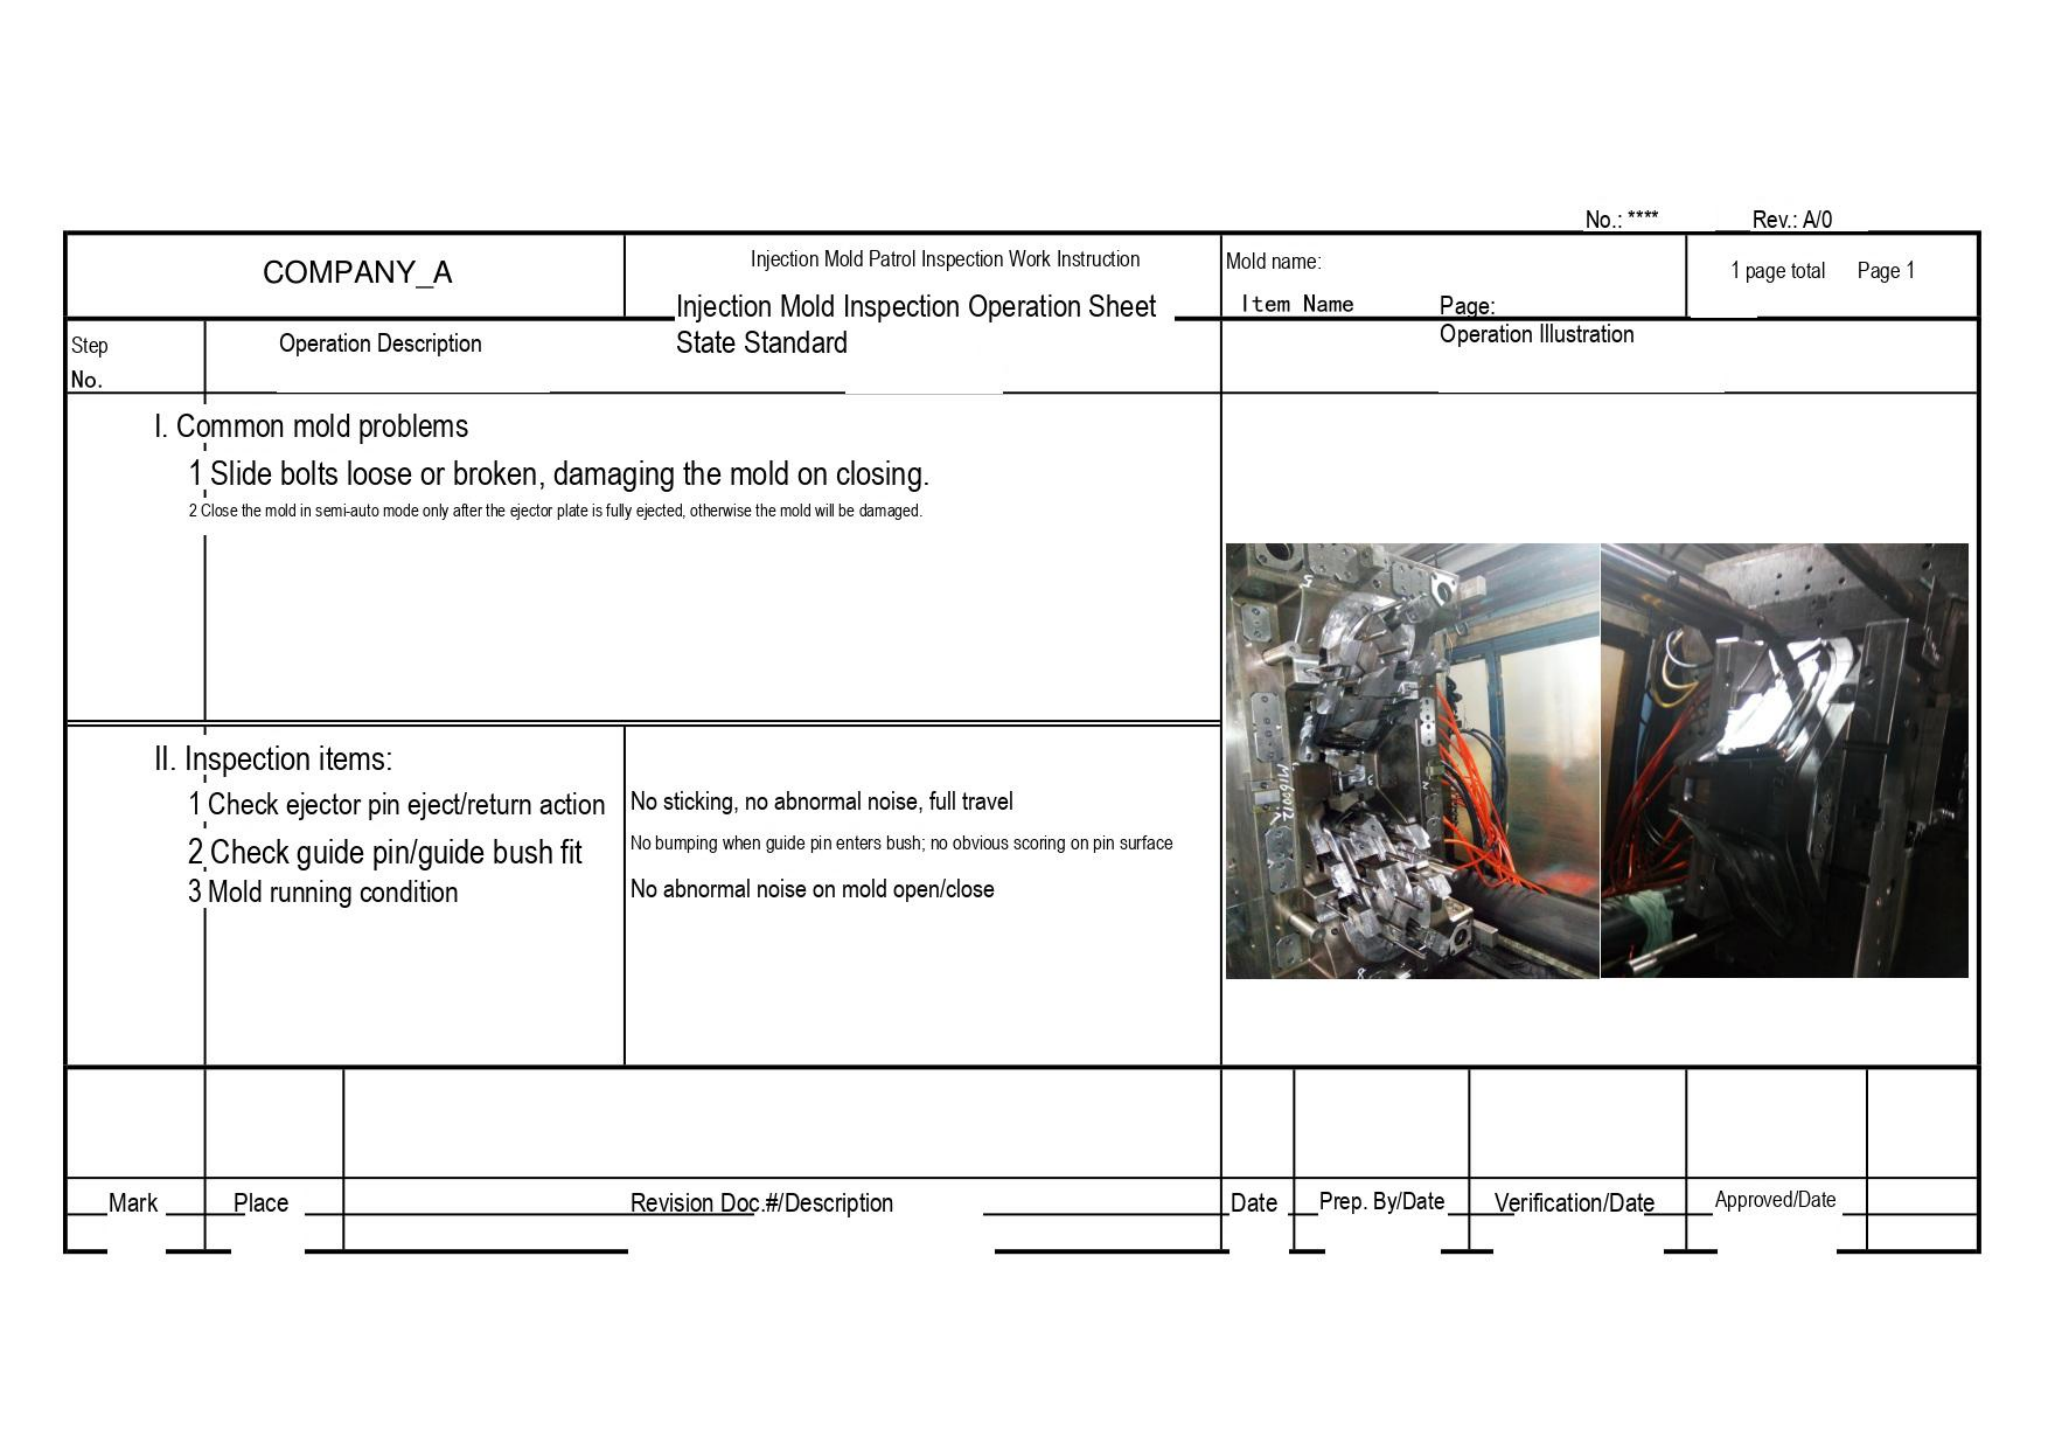No.: **** Rev.: A/0

| COMPANY_A | Injection Mold Patrol Inspection Work Instruction<br>Injection Mold Inspection Operation Sheet | Mold name:<br>Item Name Page: | 1 page total Page 1 |
|---|---|---|---|

| Step No. | Operation Description | State Standard | Operation Illustration |
|---|---|---|---|
| | I. Common mold problems<br>1 Slide bolts loose or broken, damaging the mold on closing.<br>2 Close the mold in semi-auto mode only after the ejector plate is fully ejected, otherwise the mold will be damaged. | | |
| | II. Inspection items:<br>1 Check ejector pin eject/return action | No sticking, no abnormal noise, full travel | |
| | 2 Check guide pin/guide bush fit | No bumping when guide pin enters bush; no obvious scoring on pin surface | |
| | 3 Mold running condition | No abnormal noise on mold open/close | |

| Mark | Place | Revision Doc.#/Description | Date | Prep. By/Date | Verification/Date | Approved/Date |
|---|---|---|---|---|---|---|
| | | | | | | |